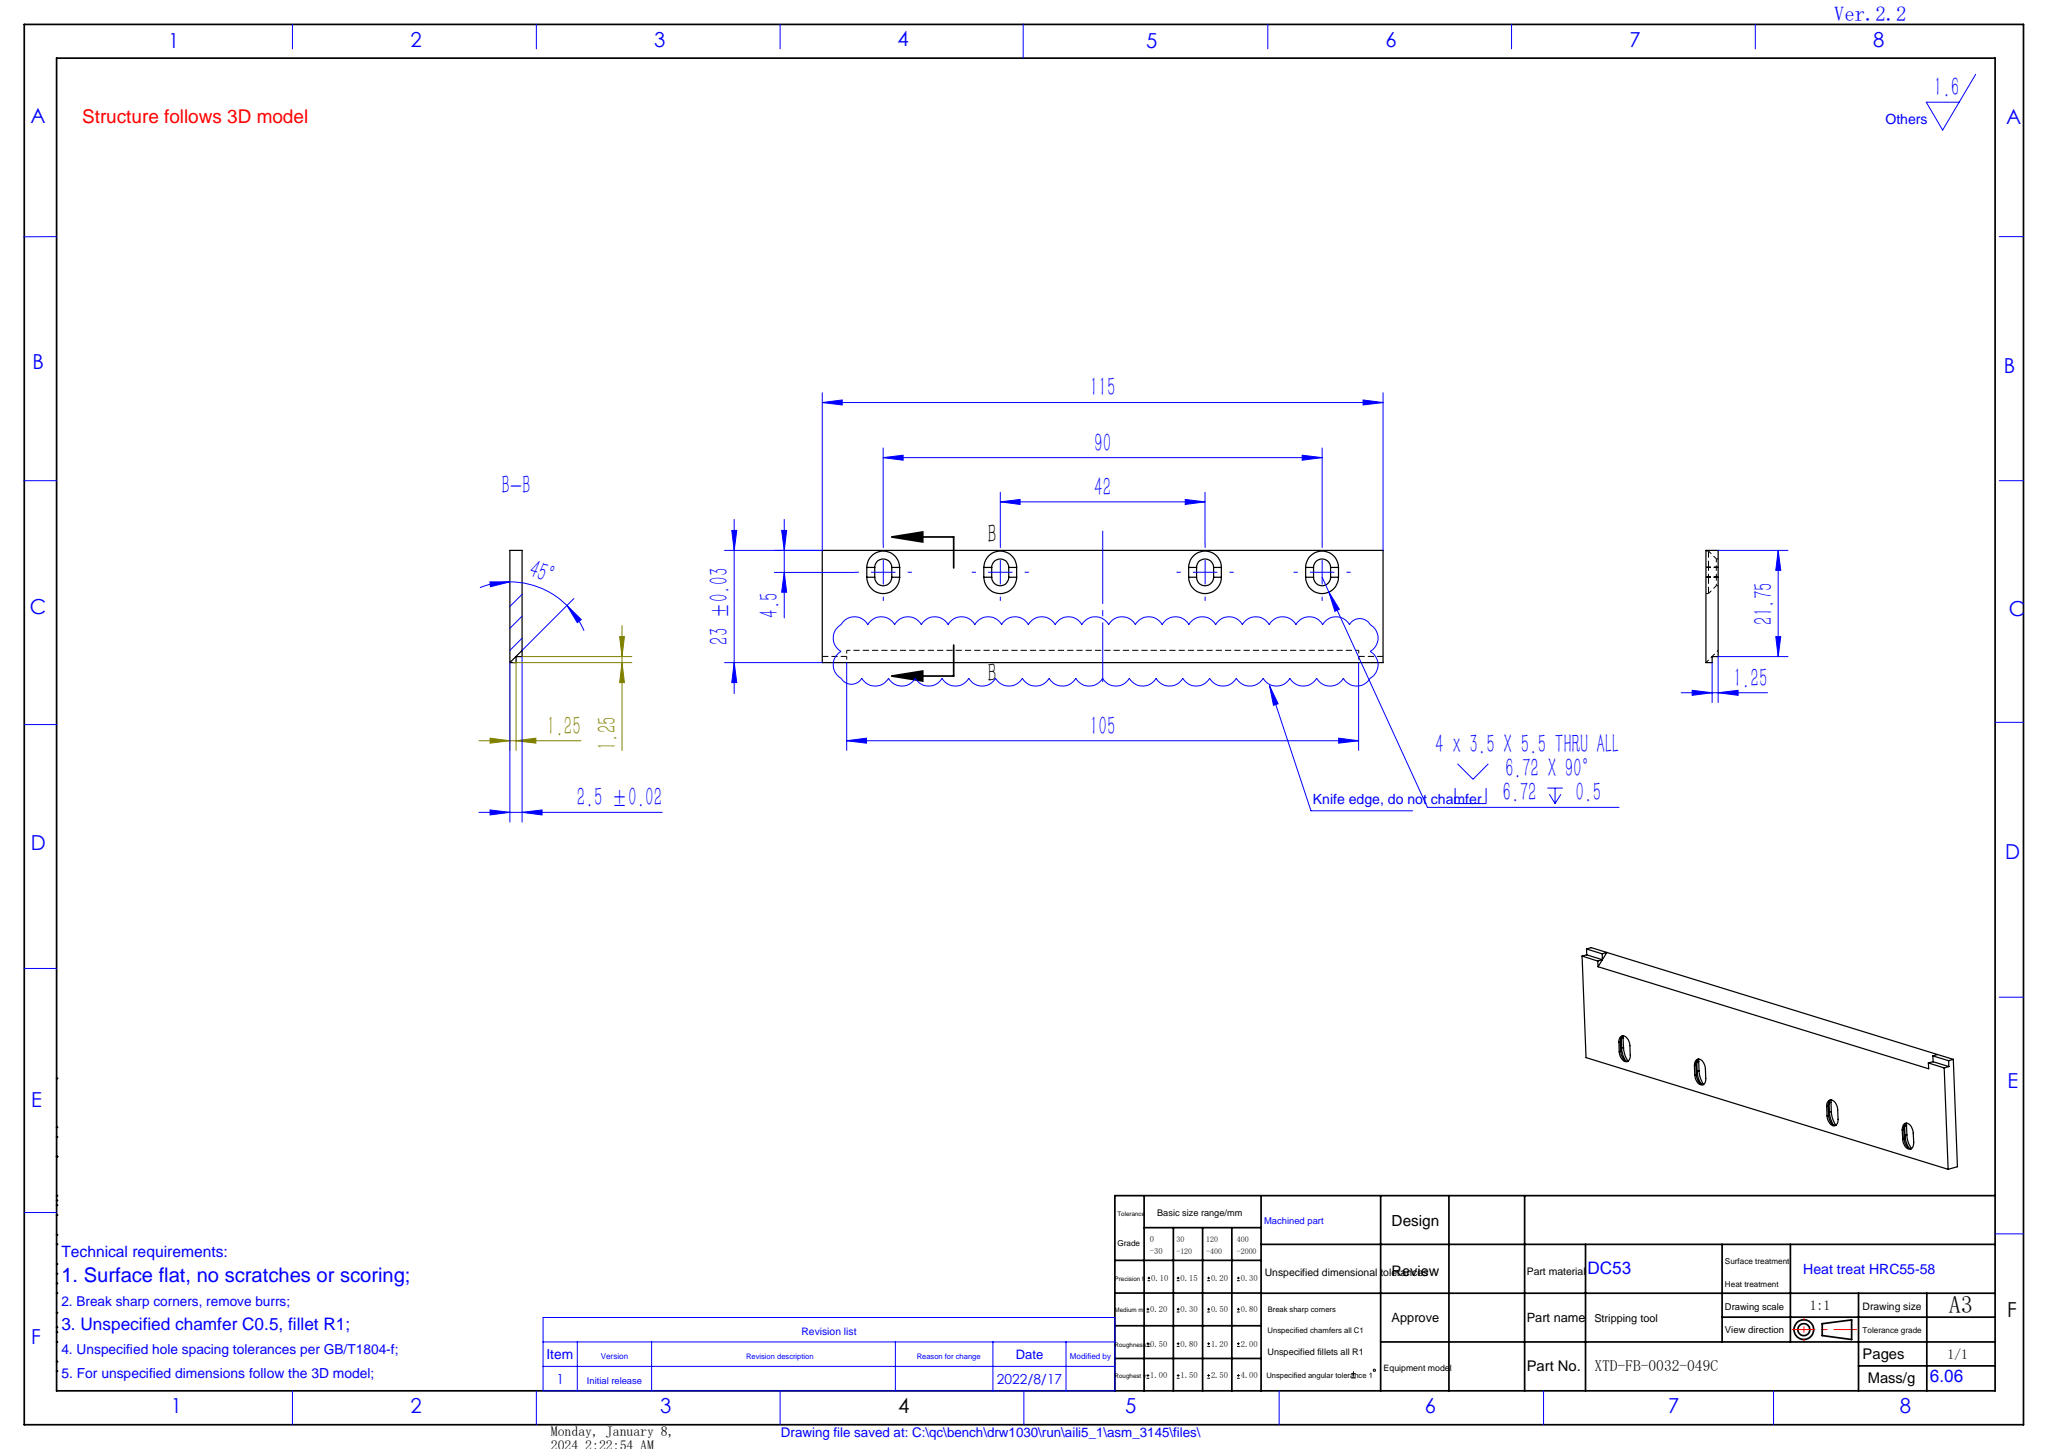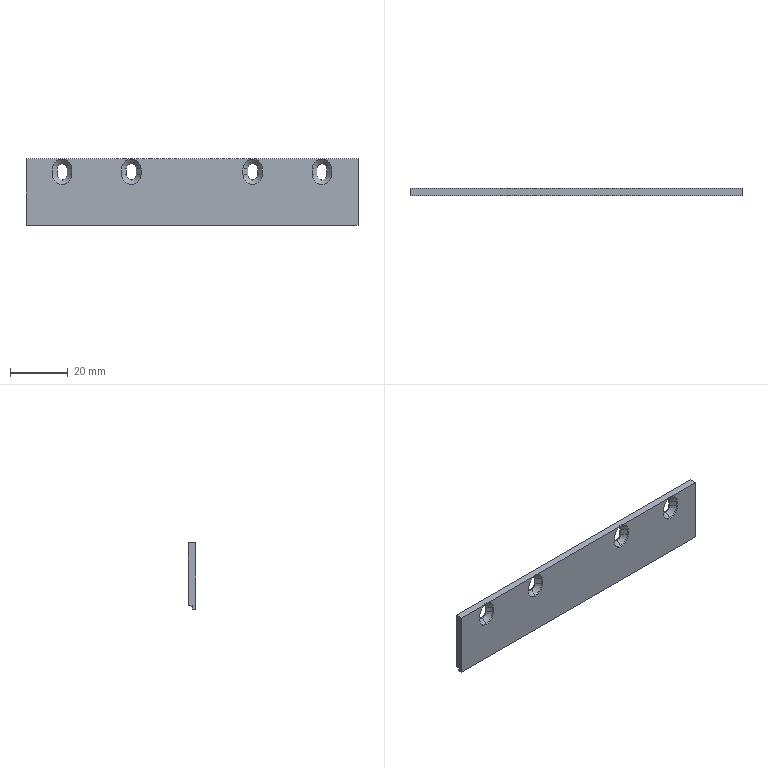Part | SolidWorks | features ICE 2, Extrusion 1, HoleWzd 1 | 1 solid | 76 faces | box 115 x 2.5 x 23 mm | volume 5943 mm3 | plane 40 | cylinder 24 | cone 12 | commonest cylinder face diameters 3.5 x12 6.72 x12